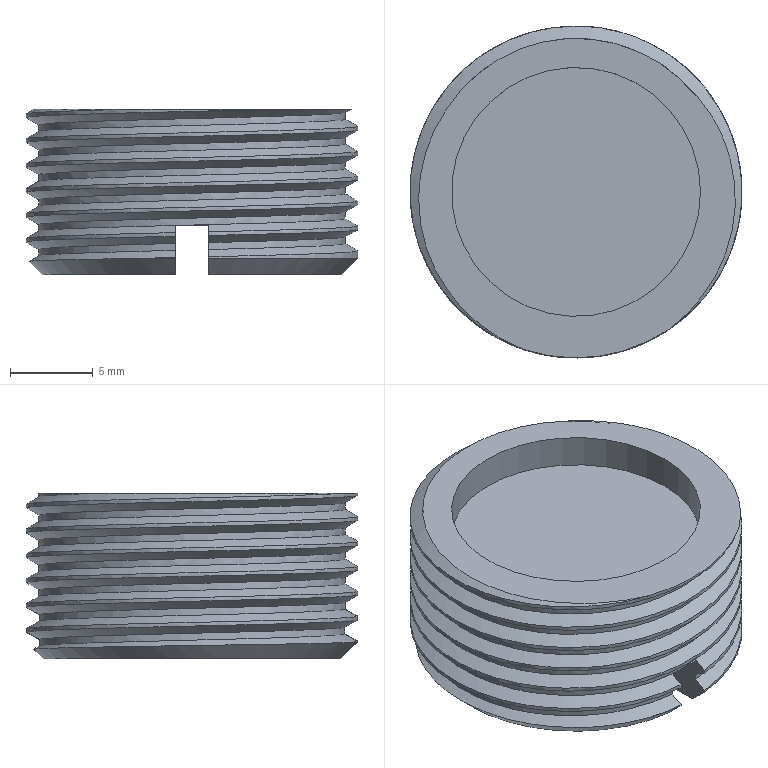Part | NX | features DATUM_CSYS 3, EXTRUDE 3, SKETCH 2, CHAMFER 1, THREADS 1 | 1 solid | 27 faces | box 20 x 20 x 10 mm | volume 2405 mm3 | cylinder 9 | plane 8 | spline 8 | cone 2 | commonest cylinder face diameters 18.5 x4 20 x4 15 x1